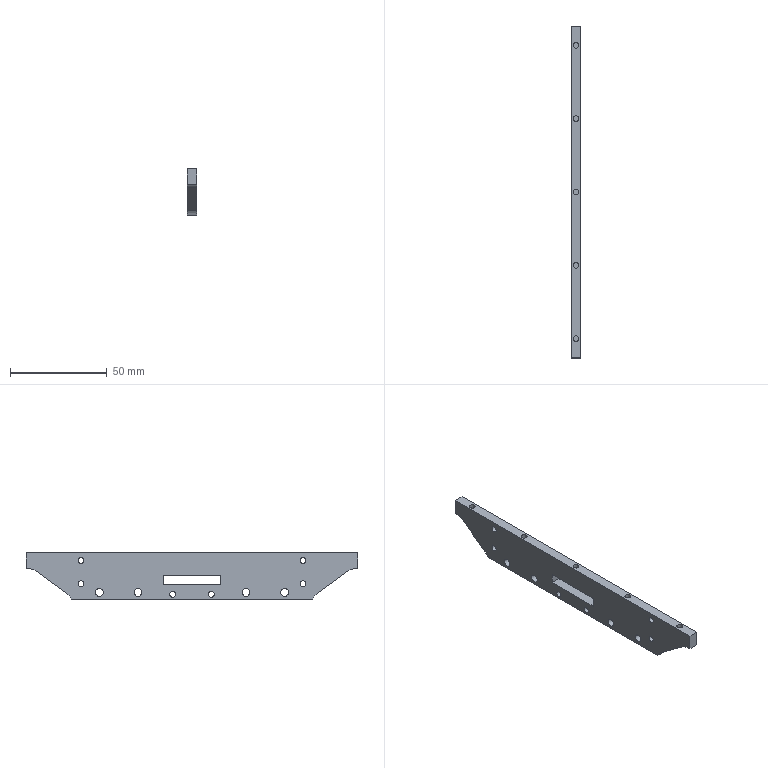Part | STEP file | 1-28.3 | 1 solid | 36 faces | box 5 x 172 x 24 mm | volume 17032 mm3 | cylinder 19 | plane 17 | commonest cylinder face diameters 3 x11 4 x4 10 x2 20 x2